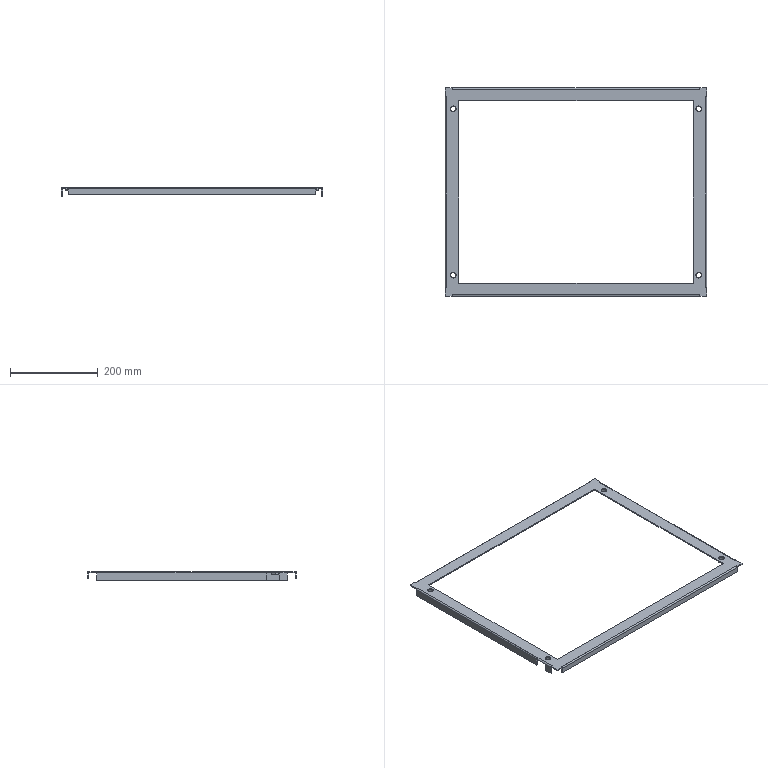Part | SolidWorks | features ICE 3, EdgeFlange 2, MirrorPattern 2, Cut 1, FlatPattern 1, LPattern 1, SMBaseFlange 1, SheetMetal 1 | 1 solid | 118 faces | box 596 x 476 x 20 mm | volume 219938 mm3 | plane 94 | cylinder 24 | commonest cylinder face diameters 12 x8 13 x8 1 x4 6 x4